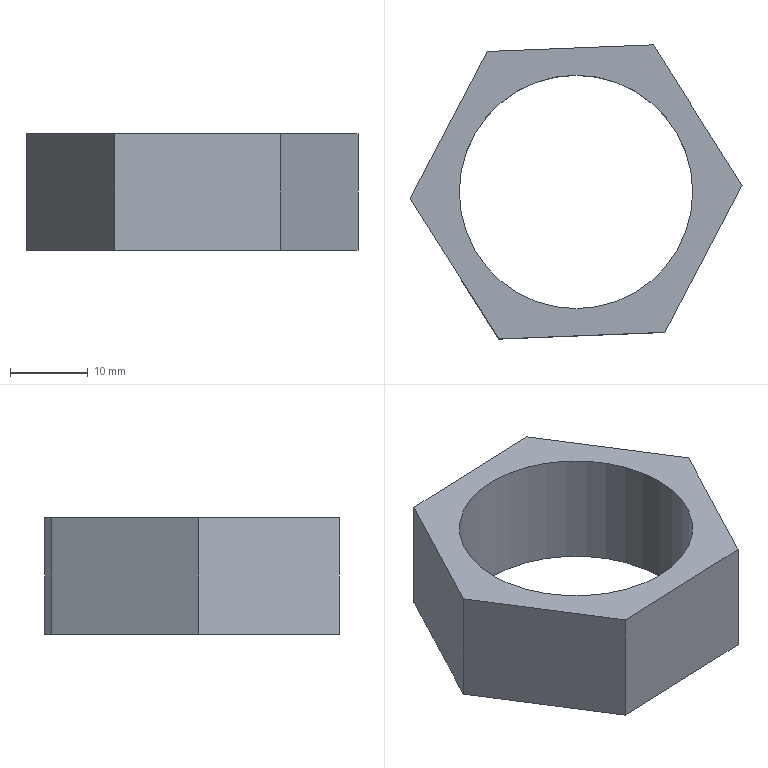Part | SolidWorks | features Extrusion 1 | 1 solid | 10 faces | box 42.69 x 37.825 x 15 mm | volume 7181 mm3 | plane 8 | cylinder 2 | commonest cylinder face diameters 30 x2
STEP:
#1=CARTESIAN_POINT('',(-15.,0.,15.));
#2=VERTEX_POINT('',#1);
#3=CARTESIAN_POINT('',(15.,0.,15.));
#4=VERTEX_POINT('',#3);
#5=CARTESIAN_POINT('',(0.,0.,15.));
#6=DIRECTION('',(0.,0.,1.));
#7=DIRECTION('',(1.,0.,0.));
#8=AXIS2_PLACEMENT_3D('',#5,#6,#7);
#9=CIRCLE('',#8,15.);
#10=EDGE_CURVE('',#2,#4,#9,.T.);
#11=ORIENTED_EDGE('',*,*,#10,.T.);
#12=CARTESIAN_POINT('',(15.,0.,0.));
#13=VERTEX_POINT('',#12);
#14=CARTESIAN_POINT('',(15.,0.,15.));
#15=DIRECTION('',(0.,0.,-1.));
#16=VECTOR('',#15,1000.);
#17=LINE('',#14,#16);
#18=EDGE_CURVE('',#4,#13,#17,.T.);
#19=ORIENTED_EDGE('',*,*,#18,.T.);
#20=CARTESIAN_POINT('',(-15.,0.,0.));
#21=VERTEX_POINT('',#20);
#22=CARTESIAN_POINT('',(0.,0.,0.));
#23=DIRECTION('',(0.,0.,1.));
#24=DIRECTION('',(1.,0.,0.));
#25=AXIS2_PLACEMENT_3D('',#22,#23,#24);
#26=CIRCLE('',#25,15.);
#27=EDGE_CURVE('',#21,#13,#26,.T.);
#28=ORIENTED_EDGE('',*,*,#27,.F.);
#29=CARTESIAN_POINT('',(-15.,0.,15.));
#30=DIRECTION('',(0.,0.,-1.));
#31=VECTOR('',#30,1000.);
#32=LINE('',#29,#31);
#33=EDGE_CURVE('',#2,#21,#32,.T.);
#34=ORIENTED_EDGE('',*,*,#33,.F.);
#35=EDGE_LOOP('',(#11,#19,#28,#34));
#36=FACE_OUTER_BOUND('',#35,.T.);
#37=CARTESIAN_POINT('',(0.,0.,15.));
#38=DIRECTION('',(0.,0.,-1.));
#39=DIRECTION('',(-1.,0.,0.));
#40=AXIS2_PLACEMENT_3D('',#37,#38,#39);
#41=CYLINDRICAL_SURFACE('',#40,15.);
#42=ADVANCED_FACE('',(#36),#41,.F.);
#43=CARTESIAN_POINT('',(21.345,0.8542,15.));
#44=VERTEX_POINT('',#43);
#45=CARTESIAN_POINT('',(9.933,18.912,15.));
#46=VERTEX_POINT('',#45);
#47=CARTESIAN_POINT('',(21.345,0.8542,15.));
#48=DIRECTION('',(-0.5342,0.8453,0.));
#49=VECTOR('',#48,1000.);
#50=LINE('',#47,#49);
#51=EDGE_CURVE('',#44,#46,#50,.T.);
#52=ORIENTED_EDGE('',*,*,#51,.T.);
#53=CARTESIAN_POINT('',(-11.412,18.058,15.));
#54=VERTEX_POINT('',#53);
#55=CARTESIAN_POINT('',(9.933,18.912,15.));
#56=DIRECTION('',(-0.9992,-0.03999,0.));
#57=VECTOR('',#56,1000.);
#58=LINE('',#55,#57);
#59=EDGE_CURVE('',#46,#54,#58,.T.);
#60=ORIENTED_EDGE('',*,*,#59,.T.);
#61=CARTESIAN_POINT('',(-21.345,-0.8542,15.));
#62=VERTEX_POINT('',#61);
#63=CARTESIAN_POINT('',(-11.412,18.058,15.));
#64=DIRECTION('',(-0.465,-0.8853,0.));
#65=VECTOR('',#64,1000.);
#66=LINE('',#63,#65);
#67=EDGE_CURVE('',#54,#62,#66,.T.);
#68=ORIENTED_EDGE('',*,*,#67,.T.);
#69=CARTESIAN_POINT('',(-9.933,-18.912,15.));
#70=VERTEX_POINT('',#69);
#71=CARTESIAN_POINT('',(-21.345,-0.8542,15.));
#72=DIRECTION('',(0.5342,-0.8453,0.));
#73=VECTOR('',#72,1000.);
#74=LINE('',#71,#73);
#75=EDGE_CURVE('',#62,#70,#74,.T.);
#76=ORIENTED_EDGE('',*,*,#75,.T.);
#77=CARTESIAN_POINT('',(11.412,-18.058,15.));
#78=VERTEX_POINT('',#77);
#79=CARTESIAN_POINT('',(-9.933,-18.912,15.));
#80=DIRECTION('',(0.9992,0.03999,0.));
#81=VECTOR('',#80,1000.);
#82=LINE('',#79,#81);
#83=EDGE_CURVE('',#70,#78,#82,.T.);
#84=ORIENTED_EDGE('',*,*,#83,.T.);
#85=CARTESIAN_POINT('',(11.412,-18.058,15.));
#86=DIRECTION('',(0.465,0.8853,0.));
#87=VECTOR('',#86,1000.);
#88=LINE('',#85,#87);
#89=EDGE_CURVE('',#78,#44,#88,.T.);
#90=ORIENTED_EDGE('',*,*,#89,.T.);
#91=EDGE_LOOP('',(#52,#60,#68,#76,#84,#90));
#92=FACE_OUTER_BOUND('',#91,.T.);
#93=ORIENTED_EDGE('',*,*,#10,.F.);
#94=CARTESIAN_POINT('',(0.,0.,15.));
#95=DIRECTION('',(0.,0.,1.));
#96=DIRECTION('',(1.,0.,0.));
#97=AXIS2_PLACEMENT_3D('',#94,#95,#96);
#98=CIRCLE('',#97,15.);
#99=EDGE_CURVE('',#4,#2,#98,.T.);
#100=ORIENTED_EDGE('',*,*,#99,.F.);
#101=EDGE_LOOP('',(#93,#100));
#102=FACE_BOUND('',#101,.T.);
#103=CARTESIAN_POINT('',(0.,0.,15.));
#104=DIRECTION('',(0.,0.,1.));
#105=DIRECTION('',(1.,0.,0.));
#106=AXIS2_PLACEMENT_3D('',#103,#104,#105);
#107=PLANE('',#106);
#108=ADVANCED_FACE('',(#92,#102),#107,.T.);
#109=CARTESIAN_POINT('',(21.345,0.8542,0.));
#110=VERTEX_POINT('',#109);
#111=CARTESIAN_POINT('',(9.933,18.912,0.));
#112=VERTEX_POINT('',#111);
#113=CARTESIAN_POINT('',(21.345,0.8542,0.));
#114=DIRECTION('',(-0.5342,0.8453,0.));
#115=VECTOR('',#114,1000.);
#116=LINE('',#113,#115);
#117=EDGE_CURVE('',#110,#112,#116,.T.);
#118=ORIENTED_EDGE('',*,*,#117,.F.);
#119=CARTESIAN_POINT('',(11.412,-18.058,0.));
#120=VERTEX_POINT('',#119);
#121=CARTESIAN_POINT('',(11.412,-18.058,0.));
#122=DIRECTION('',(0.465,0.8853,0.));
#123=VECTOR('',#122,1000.);
#124=LINE('',#121,#123);
#125=EDGE_CURVE('',#120,#110,#124,.T.);
#126=ORIENTED_EDGE('',*,*,#125,.F.);
#127=CARTESIAN_POINT('',(-9.933,-18.912,0.));
#128=VERTEX_POINT('',#127);
#129=CARTESIAN_POINT('',(-9.933,-18.912,0.));
#130=DIRECTION('',(0.9992,0.03999,0.));
#131=VECTOR('',#130,1000.);
#132=LINE('',#129,#131);
#133=EDGE_CURVE('',#128,#120,#132,.T.);
#134=ORIENTED_EDGE('',*,*,#133,.F.);
#135=CARTESIAN_POINT('',(-21.345,-0.8542,0.));
#136=VERTEX_POINT('',#135);
#137=CARTESIAN_POINT('',(-21.345,-0.8542,0.));
#138=DIRECTION('',(0.5342,-0.8453,0.));
#139=VECTOR('',#138,1000.);
#140=LINE('',#137,#139);
#141=EDGE_CURVE('',#136,#128,#140,.T.);
#142=ORIENTED_EDGE('',*,*,#141,.F.);
#143=CARTESIAN_POINT('',(-11.412,18.058,0.));
#144=VERTEX_POINT('',#143);
#145=CARTESIAN_POINT('',(-11.412,18.058,0.));
#146=DIRECTION('',(-0.465,-0.8853,0.));
#147=VECTOR('',#146,1000.);
#148=LINE('',#145,#147);
#149=EDGE_CURVE('',#144,#136,#148,.T.);
#150=ORIENTED_EDGE('',*,*,#149,.F.);
#151=CARTESIAN_POINT('',(9.933,18.912,0.));
#152=DIRECTION('',(-0.9992,-0.03999,0.));
#153=VECTOR('',#152,1000.);
#154=LINE('',#151,#153);
#155=EDGE_CURVE('',#112,#144,#154,.T.);
#156=ORIENTED_EDGE('',*,*,#155,.F.);
#157=EDGE_LOOP('',(#118,#126,#134,#142,#150,#156));
#158=FACE_OUTER_BOUND('',#157,.T.);
#159=ORIENTED_EDGE('',*,*,#27,.T.);
#160=CARTESIAN_POINT('',(0.,0.,0.));
#161=DIRECTION('',(0.,0.,1.));
#162=DIRECTION('',(1.,0.,0.));
#163=AXIS2_PLACEMENT_3D('',#160,#161,#162);
#164=CIRCLE('',#163,15.);
#165=EDGE_CURVE('',#13,#21,#164,.T.);
#166=ORIENTED_EDGE('',*,*,#165,.T.);
#167=EDGE_LOOP('',(#159,#166));
#168=FACE_BOUND('',#167,.T.);
#169=CARTESIAN_POINT('',(0.,0.,0.));
#170=DIRECTION('',(0.,0.,1.));
#171=DIRECTION('',(1.,0.,0.));
#172=AXIS2_PLACEMENT_3D('',#169,#170,#171);
#173=PLANE('',#172);
#174=ADVANCED_FACE('',(#158,#168),#173,.F.);
#175=ORIENTED_EDGE('',*,*,#117,.T.);
#176=CARTESIAN_POINT('',(9.933,18.912,15.));
#177=DIRECTION('',(0.,0.,-1.));
#178=VECTOR('',#177,1000.);
#179=LINE('',#176,#178);
#180=EDGE_CURVE('',#46,#112,#179,.T.);
#181=ORIENTED_EDGE('',*,*,#180,.F.);
#182=ORIENTED_EDGE('',*,*,#51,.F.);
#183=CARTESIAN_POINT('',(21.345,0.8542,15.));
#184=DIRECTION('',(0.,0.,-1.));
#185=VECTOR('',#184,1000.);
#186=LINE('',#183,#185);
#187=EDGE_CURVE('',#44,#110,#186,.T.);
#188=ORIENTED_EDGE('',*,*,#187,.T.);
#189=EDGE_LOOP('',(#175,#181,#182,#188));
#190=FACE_OUTER_BOUND('',#189,.T.);
#191=CARTESIAN_POINT('',(21.345,0.8542,15.));
#192=DIRECTION('',(-0.8453,-0.5342,0.));
#193=DIRECTION('',(0.5342,-0.8453,0.));
#194=AXIS2_PLACEMENT_3D('',#191,#192,#193);
#195=PLANE('',#194);
#196=ADVANCED_FACE('',(#190),#195,.F.);
#197=ORIENTED_EDGE('',*,*,#155,.T.);
#198=CARTESIAN_POINT('',(-11.412,18.058,15.));
#199=DIRECTION('',(0.,0.,-1.));
#200=VECTOR('',#199,1000.);
#201=LINE('',#198,#200);
#202=EDGE_CURVE('',#54,#144,#201,.T.);
#203=ORIENTED_EDGE('',*,*,#202,.F.);
#204=ORIENTED_EDGE('',*,*,#59,.F.);
#205=ORIENTED_EDGE('',*,*,#180,.T.);
#206=EDGE_LOOP('',(#197,#203,#204,#205));
#207=FACE_OUTER_BOUND('',#206,.T.);
#208=CARTESIAN_POINT('',(9.933,18.912,15.));
#209=DIRECTION('',(0.03999,-0.9992,0.));
#210=DIRECTION('',(0.9992,0.03999,0.));
#211=AXIS2_PLACEMENT_3D('',#208,#209,#210);
#212=PLANE('',#211);
#213=ADVANCED_FACE('',(#207),#212,.F.);
#214=ORIENTED_EDGE('',*,*,#149,.T.);
#215=CARTESIAN_POINT('',(-21.345,-0.8542,15.));
#216=DIRECTION('',(0.,0.,-1.));
#217=VECTOR('',#216,1000.);
#218=LINE('',#215,#217);
#219=EDGE_CURVE('',#62,#136,#218,.T.);
#220=ORIENTED_EDGE('',*,*,#219,.F.);
#221=ORIENTED_EDGE('',*,*,#67,.F.);
#222=ORIENTED_EDGE('',*,*,#202,.T.);
#223=EDGE_LOOP('',(#214,#220,#221,#222));
#224=FACE_OUTER_BOUND('',#223,.T.);
#225=CARTESIAN_POINT('',(-11.412,18.058,15.));
#226=DIRECTION('',(0.8853,-0.465,0.));
#227=DIRECTION('',(0.465,0.8853,0.));
#228=AXIS2_PLACEMENT_3D('',#225,#226,#227);
#229=PLANE('',#228);
#230=ADVANCED_FACE('',(#224),#229,.F.);
#231=ORIENTED_EDGE('',*,*,#141,.T.);
#232=CARTESIAN_POINT('',(-9.933,-18.912,15.));
#233=DIRECTION('',(0.,0.,-1.));
#234=VECTOR('',#233,1000.);
#235=LINE('',#232,#234);
#236=EDGE_CURVE('',#70,#128,#235,.T.);
#237=ORIENTED_EDGE('',*,*,#236,.F.);
#238=ORIENTED_EDGE('',*,*,#75,.F.);
#239=ORIENTED_EDGE('',*,*,#219,.T.);
#240=EDGE_LOOP('',(#231,#237,#238,#239));
#241=FACE_OUTER_BOUND('',#240,.T.);
#242=CARTESIAN_POINT('',(-21.345,-0.8542,15.));
#243=DIRECTION('',(0.8453,0.5342,0.));
#244=DIRECTION('',(-0.5342,0.8453,0.));
#245=AXIS2_PLACEMENT_3D('',#242,#243,#244);
#246=PLANE('',#245);
#247=ADVANCED_FACE('',(#241),#246,.F.);
#248=ORIENTED_EDGE('',*,*,#133,.T.);
#249=CARTESIAN_POINT('',(11.412,-18.058,15.));
#250=DIRECTION('',(0.,0.,-1.));
#251=VECTOR('',#250,1000.);
#252=LINE('',#249,#251);
#253=EDGE_CURVE('',#78,#120,#252,.T.);
#254=ORIENTED_EDGE('',*,*,#253,.F.);
#255=ORIENTED_EDGE('',*,*,#83,.F.);
#256=ORIENTED_EDGE('',*,*,#236,.T.);
#257=EDGE_LOOP('',(#248,#254,#255,#256));
#258=FACE_OUTER_BOUND('',#257,.T.);
#259=CARTESIAN_POINT('',(-9.933,-18.912,15.));
#260=DIRECTION('',(-0.03999,0.9992,0.));
#261=DIRECTION('',(-0.9992,-0.03999,0.));
#262=AXIS2_PLACEMENT_3D('',#259,#260,#261);
#263=PLANE('',#262);
#264=ADVANCED_FACE('',(#258),#263,.F.);
#265=ORIENTED_EDGE('',*,*,#125,.T.);
#266=ORIENTED_EDGE('',*,*,#187,.F.);
#267=ORIENTED_EDGE('',*,*,#89,.F.);
#268=ORIENTED_EDGE('',*,*,#253,.T.);
#269=EDGE_LOOP('',(#265,#266,#267,#268));
#270=FACE_OUTER_BOUND('',#269,.T.);
#271=CARTESIAN_POINT('',(11.412,-18.058,15.));
#272=DIRECTION('',(-0.8853,0.465,0.));
#273=DIRECTION('',(-0.465,-0.8853,0.));
#274=AXIS2_PLACEMENT_3D('',#271,#272,#273);
#275=PLANE('',#274);
#276=ADVANCED_FACE('',(#270),#275,.F.);
#277=ORIENTED_EDGE('',*,*,#18,.F.);
#278=ORIENTED_EDGE('',*,*,#99,.T.);
#279=ORIENTED_EDGE('',*,*,#33,.T.);
#280=ORIENTED_EDGE('',*,*,#165,.F.);
#281=EDGE_LOOP('',(#277,#278,#279,#280));
#282=FACE_OUTER_BOUND('',#281,.T.);
#283=CARTESIAN_POINT('',(0.,0.,15.));
#284=DIRECTION('',(0.,0.,-1.));
#285=DIRECTION('',(-1.,0.,0.));
#286=AXIS2_PLACEMENT_3D('',#283,#284,#285);
#287=CYLINDRICAL_SURFACE('',#286,15.);
#288=ADVANCED_FACE('',(#282),#287,.F.);
#289=CLOSED_SHELL('',(#42,#108,#174,#196,#213,#230,#247,#264,#276,#288));
#290=MANIFOLD_SOLID_BREP('',#289);
#291=CARTESIAN_POINT('',(0.,0.,0.));
#292=DIRECTION('',(0.,0.,1.));
#293=DIRECTION('',(1.,0.,0.));
#294=AXIS2_PLACEMENT_3D('',#291,#292,#293);
#295=(LENGTH_UNIT()NAMED_UNIT(*)SI_UNIT(.MILLI.,.METRE.));
#296=UNCERTAINTY_MEASURE_WITH_UNIT(LENGTH_MEASURE(0.00001),#295,'','');
#297=(NAMED_UNIT(*)PLANE_ANGLE_UNIT()SI_UNIT($,.RADIAN.));
#298=(NAMED_UNIT(*)SI_UNIT($,.STERADIAN.)SOLID_ANGLE_UNIT());
#299=(GEOMETRIC_REPRESENTATION_CONTEXT(3)GLOBAL_UNCERTAINTY_ASSIGNED_CONTEXT((#296))GLOBAL_UNIT_ASSIGNED_CONTEXT((#295,#297,#298))REPRESENTATION_CONTEXT('',''));
#300=ADVANCED_BREP_SHAPE_REPRESENTATION('',(#290,#294),#299);